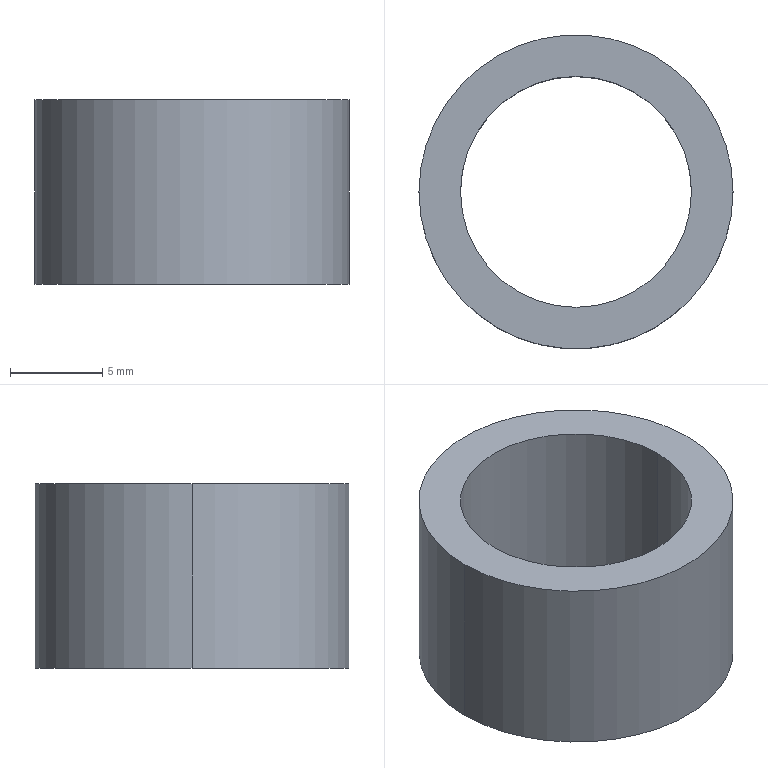Part | SolidWorks | features Extrusion 1 | 1 solid | 6 faces | box 17 x 17 x 10 mm | volume 1043 mm3 | cylinder 4 | plane 2 | commonest cylinder face diameters 12.5 x2 17 x2
STEP:
#1=CARTESIAN_POINT('',(-6.25,0.,10.));
#2=VERTEX_POINT('',#1);
#3=CARTESIAN_POINT('',(6.25,0.,10.));
#4=VERTEX_POINT('',#3);
#5=CARTESIAN_POINT('',(0.,0.,10.));
#6=DIRECTION('',(0.,0.,1.));
#7=DIRECTION('',(1.,0.,0.));
#8=AXIS2_PLACEMENT_3D('',#5,#6,#7);
#9=CIRCLE('',#8,6.25);
#10=EDGE_CURVE('',#2,#4,#9,.T.);
#11=ORIENTED_EDGE('',*,*,#10,.T.);
#12=CARTESIAN_POINT('',(6.25,0.,0.));
#13=VERTEX_POINT('',#12);
#14=CARTESIAN_POINT('',(6.25,0.,10.));
#15=DIRECTION('',(0.,0.,-1.));
#16=VECTOR('',#15,1000.);
#17=LINE('',#14,#16);
#18=EDGE_CURVE('',#4,#13,#17,.T.);
#19=ORIENTED_EDGE('',*,*,#18,.T.);
#20=CARTESIAN_POINT('',(-6.25,0.,0.));
#21=VERTEX_POINT('',#20);
#22=CARTESIAN_POINT('',(0.,0.,0.));
#23=DIRECTION('',(0.,0.,1.));
#24=DIRECTION('',(1.,0.,0.));
#25=AXIS2_PLACEMENT_3D('',#22,#23,#24);
#26=CIRCLE('',#25,6.25);
#27=EDGE_CURVE('',#21,#13,#26,.T.);
#28=ORIENTED_EDGE('',*,*,#27,.F.);
#29=CARTESIAN_POINT('',(-6.25,0.,10.));
#30=DIRECTION('',(0.,0.,-1.));
#31=VECTOR('',#30,1000.);
#32=LINE('',#29,#31);
#33=EDGE_CURVE('',#2,#21,#32,.T.);
#34=ORIENTED_EDGE('',*,*,#33,.F.);
#35=EDGE_LOOP('',(#11,#19,#28,#34));
#36=FACE_OUTER_BOUND('',#35,.T.);
#37=CARTESIAN_POINT('',(0.,0.,10.));
#38=DIRECTION('',(0.,0.,-1.));
#39=DIRECTION('',(-1.,0.,0.));
#40=AXIS2_PLACEMENT_3D('',#37,#38,#39);
#41=CYLINDRICAL_SURFACE('',#40,6.25);
#42=ADVANCED_FACE('',(#36),#41,.F.);
#43=CARTESIAN_POINT('',(8.5,0.,10.));
#44=VERTEX_POINT('',#43);
#45=CARTESIAN_POINT('',(-8.5,0.,10.));
#46=VERTEX_POINT('',#45);
#47=CARTESIAN_POINT('',(0.,0.,10.));
#48=DIRECTION('',(0.,0.,1.));
#49=DIRECTION('',(1.,0.,0.));
#50=AXIS2_PLACEMENT_3D('',#47,#48,#49);
#51=CIRCLE('',#50,8.5);
#52=EDGE_CURVE('',#44,#46,#51,.T.);
#53=ORIENTED_EDGE('',*,*,#52,.F.);
#54=CARTESIAN_POINT('',(8.5,0.,0.));
#55=VERTEX_POINT('',#54);
#56=CARTESIAN_POINT('',(8.5,0.,10.));
#57=DIRECTION('',(0.,0.,-1.));
#58=VECTOR('',#57,1000.);
#59=LINE('',#56,#58);
#60=EDGE_CURVE('',#44,#55,#59,.T.);
#61=ORIENTED_EDGE('',*,*,#60,.T.);
#62=CARTESIAN_POINT('',(-8.5,0.,0.));
#63=VERTEX_POINT('',#62);
#64=CARTESIAN_POINT('',(0.,0.,0.));
#65=DIRECTION('',(0.,0.,1.));
#66=DIRECTION('',(1.,0.,0.));
#67=AXIS2_PLACEMENT_3D('',#64,#65,#66);
#68=CIRCLE('',#67,8.5);
#69=EDGE_CURVE('',#55,#63,#68,.T.);
#70=ORIENTED_EDGE('',*,*,#69,.T.);
#71=CARTESIAN_POINT('',(-8.5,0.,10.));
#72=DIRECTION('',(0.,0.,-1.));
#73=VECTOR('',#72,1000.);
#74=LINE('',#71,#73);
#75=EDGE_CURVE('',#46,#63,#74,.T.);
#76=ORIENTED_EDGE('',*,*,#75,.F.);
#77=EDGE_LOOP('',(#53,#61,#70,#76));
#78=FACE_OUTER_BOUND('',#77,.T.);
#79=CARTESIAN_POINT('',(0.,0.,10.));
#80=DIRECTION('',(0.,0.,-1.));
#81=DIRECTION('',(-1.,0.,0.));
#82=AXIS2_PLACEMENT_3D('',#79,#80,#81);
#83=CYLINDRICAL_SURFACE('',#82,8.5);
#84=ADVANCED_FACE('',(#78),#83,.T.);
#85=CARTESIAN_POINT('',(0.,0.,10.));
#86=DIRECTION('',(0.,0.,1.));
#87=DIRECTION('',(1.,0.,0.));
#88=AXIS2_PLACEMENT_3D('',#85,#86,#87);
#89=CIRCLE('',#88,8.5);
#90=EDGE_CURVE('',#46,#44,#89,.T.);
#91=ORIENTED_EDGE('',*,*,#90,.T.);
#92=ORIENTED_EDGE('',*,*,#52,.T.);
#93=EDGE_LOOP('',(#91,#92));
#94=FACE_OUTER_BOUND('',#93,.T.);
#95=ORIENTED_EDGE('',*,*,#10,.F.);
#96=CARTESIAN_POINT('',(0.,0.,10.));
#97=DIRECTION('',(0.,0.,1.));
#98=DIRECTION('',(1.,0.,0.));
#99=AXIS2_PLACEMENT_3D('',#96,#97,#98);
#100=CIRCLE('',#99,6.25);
#101=EDGE_CURVE('',#4,#2,#100,.T.);
#102=ORIENTED_EDGE('',*,*,#101,.F.);
#103=EDGE_LOOP('',(#95,#102));
#104=FACE_BOUND('',#103,.T.);
#105=CARTESIAN_POINT('',(0.,0.,10.));
#106=DIRECTION('',(0.,0.,1.));
#107=DIRECTION('',(1.,0.,0.));
#108=AXIS2_PLACEMENT_3D('',#105,#106,#107);
#109=PLANE('',#108);
#110=ADVANCED_FACE('',(#94,#104),#109,.T.);
#111=CARTESIAN_POINT('',(0.,0.,0.));
#112=DIRECTION('',(0.,0.,1.));
#113=DIRECTION('',(1.,0.,0.));
#114=AXIS2_PLACEMENT_3D('',#111,#112,#113);
#115=CIRCLE('',#114,8.5);
#116=EDGE_CURVE('',#63,#55,#115,.T.);
#117=ORIENTED_EDGE('',*,*,#116,.F.);
#118=ORIENTED_EDGE('',*,*,#69,.F.);
#119=EDGE_LOOP('',(#117,#118));
#120=FACE_OUTER_BOUND('',#119,.T.);
#121=ORIENTED_EDGE('',*,*,#27,.T.);
#122=CARTESIAN_POINT('',(0.,0.,0.));
#123=DIRECTION('',(0.,0.,1.));
#124=DIRECTION('',(1.,0.,0.));
#125=AXIS2_PLACEMENT_3D('',#122,#123,#124);
#126=CIRCLE('',#125,6.25);
#127=EDGE_CURVE('',#13,#21,#126,.T.);
#128=ORIENTED_EDGE('',*,*,#127,.T.);
#129=EDGE_LOOP('',(#121,#128));
#130=FACE_BOUND('',#129,.T.);
#131=CARTESIAN_POINT('',(0.,0.,0.));
#132=DIRECTION('',(0.,0.,1.));
#133=DIRECTION('',(1.,0.,0.));
#134=AXIS2_PLACEMENT_3D('',#131,#132,#133);
#135=PLANE('',#134);
#136=ADVANCED_FACE('',(#120,#130),#135,.F.);
#137=ORIENTED_EDGE('',*,*,#60,.F.);
#138=ORIENTED_EDGE('',*,*,#90,.F.);
#139=ORIENTED_EDGE('',*,*,#75,.T.);
#140=ORIENTED_EDGE('',*,*,#116,.T.);
#141=EDGE_LOOP('',(#137,#138,#139,#140));
#142=FACE_OUTER_BOUND('',#141,.T.);
#143=CARTESIAN_POINT('',(0.,0.,10.));
#144=DIRECTION('',(0.,0.,-1.));
#145=DIRECTION('',(-1.,0.,0.));
#146=AXIS2_PLACEMENT_3D('',#143,#144,#145);
#147=CYLINDRICAL_SURFACE('',#146,8.5);
#148=ADVANCED_FACE('',(#142),#147,.T.);
#149=ORIENTED_EDGE('',*,*,#18,.F.);
#150=ORIENTED_EDGE('',*,*,#101,.T.);
#151=ORIENTED_EDGE('',*,*,#33,.T.);
#152=ORIENTED_EDGE('',*,*,#127,.F.);
#153=EDGE_LOOP('',(#149,#150,#151,#152));
#154=FACE_OUTER_BOUND('',#153,.T.);
#155=CARTESIAN_POINT('',(0.,0.,10.));
#156=DIRECTION('',(0.,0.,-1.));
#157=DIRECTION('',(-1.,0.,0.));
#158=AXIS2_PLACEMENT_3D('',#155,#156,#157);
#159=CYLINDRICAL_SURFACE('',#158,6.25);
#160=ADVANCED_FACE('',(#154),#159,.F.);
#161=CLOSED_SHELL('',(#42,#84,#110,#136,#148,#160));
#162=MANIFOLD_SOLID_BREP('',#161);
#163=CARTESIAN_POINT('',(0.,0.,0.));
#164=DIRECTION('',(0.,0.,1.));
#165=DIRECTION('',(1.,0.,0.));
#166=AXIS2_PLACEMENT_3D('',#163,#164,#165);
#167=(LENGTH_UNIT()NAMED_UNIT(*)SI_UNIT(.MILLI.,.METRE.));
#168=UNCERTAINTY_MEASURE_WITH_UNIT(LENGTH_MEASURE(0.00001),#167,'','');
#169=(NAMED_UNIT(*)PLANE_ANGLE_UNIT()SI_UNIT($,.RADIAN.));
#170=(NAMED_UNIT(*)SI_UNIT($,.STERADIAN.)SOLID_ANGLE_UNIT());
#171=(GEOMETRIC_REPRESENTATION_CONTEXT(3)GLOBAL_UNCERTAINTY_ASSIGNED_CONTEXT((#168))GLOBAL_UNIT_ASSIGNED_CONTEXT((#167,#169,#170))REPRESENTATION_CONTEXT('',''));
#172=ADVANCED_BREP_SHAPE_REPRESENTATION('',(#162,#166),#171);